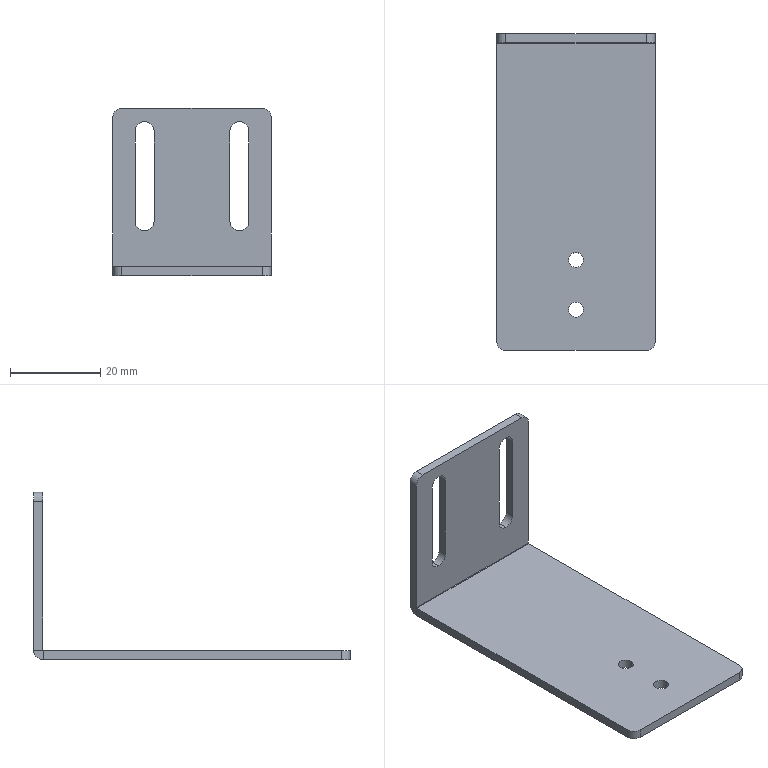Part | STEP file | 1 solid | 32 faces | box 35 x 70 x 37 mm | volume 6884 mm3 | cylinder 16 | plane 16 | commonest cylinder face diameters 4.2 x7 3.3 x4 4 x4 0.2 x1